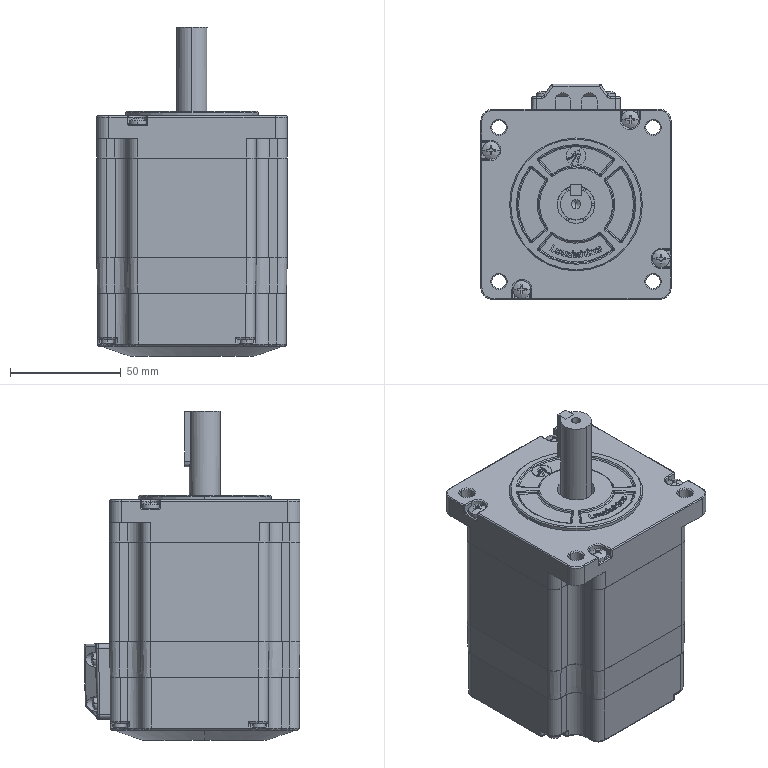Part | STEP file | 001-010-Leadshine 86CME45 (closed loop) | 30 solids | 1704 faces | box 86 x 97.458 x 148.7 mm | volume 429734 mm3 | plane 715 | cylinder 629 | spline 320 | cone 40 | commonest cylinder face diameters 2 x167 0.6 x74 1 x52 3 x32 4 x28 9 x28